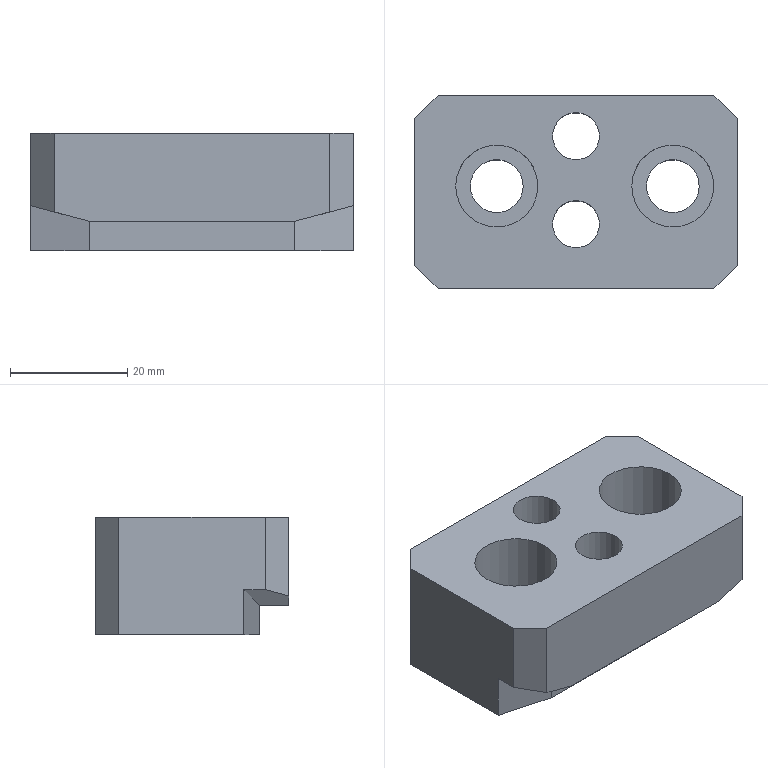Part | NX | features 20 2 | 1 solid | 24 faces | box 55 x 33 x 20 mm | volume 27724 mm3 | plane 18 | cylinder 6 | commonest cylinder face diameters 8.001 x2 9 x2 14 x2
STEP:
#1=CARTESIAN_POINT('',(974.002,435.,-3.5));
#2=VERTEX_POINT('',#1);
#3=CARTESIAN_POINT('',(969.502,435.,-3.5));
#4=DIRECTION('',(0.,0.,-1.));
#5=DIRECTION('',(1.,0.,0.));
#6=AXIS2_PLACEMENT_3D('',#3,#4,#5);
#7=CIRCLE('',#6,4.5);
#8=EDGE_CURVE('',#2,#2,#7,.T.);
#9=ORIENTED_EDGE('',*,*,#8,.F.);
#10=EDGE_LOOP('',(#9));
#11=FACE_BOUND('',#10,.T.);
#12=CARTESIAN_POINT('',(944.002,435.,-3.5));
#13=VERTEX_POINT('',#12);
#14=CARTESIAN_POINT('',(939.502,435.,-3.5));
#15=DIRECTION('',(0.,0.,1.));
#16=DIRECTION('',(1.,0.,0.));
#17=AXIS2_PLACEMENT_3D('',#14,#15,#16);
#18=CIRCLE('',#17,4.5);
#19=EDGE_CURVE('',#13,#13,#18,.T.);
#20=ORIENTED_EDGE('',*,*,#19,.T.);
#21=EDGE_LOOP('',(#20));
#22=FACE_BOUND('',#21,.T.);
#23=CARTESIAN_POINT('',(980.502,425.18,-3.5));
#24=VERTEX_POINT('',#23);
#25=CARTESIAN_POINT('',(970.501,422.5,-3.5));
#26=VERTEX_POINT('',#25);
#27=CARTESIAN_POINT('',(980.502,425.18,-3.5));
#28=DIRECTION('',(-0.9659,-0.2588,0.));
#29=VECTOR('',#28,1000.);
#30=LINE('',#27,#29);
#31=EDGE_CURVE('',#24,#26,#30,.T.);
#32=ORIENTED_EDGE('',*,*,#31,.T.);
#33=CARTESIAN_POINT('',(935.501,422.5,-3.5));
#34=VERTEX_POINT('',#33);
#35=CARTESIAN_POINT('',(981.501,422.5,-3.5));
#36=DIRECTION('',(-1.,0.,0.));
#37=VECTOR('',#36,1000.);
#38=LINE('',#35,#37);
#39=EDGE_CURVE('',#26,#34,#38,.T.);
#40=ORIENTED_EDGE('',*,*,#39,.T.);
#41=CARTESIAN_POINT('',(925.502,425.179,-3.5));
#42=VERTEX_POINT('',#41);
#43=CARTESIAN_POINT('',(935.501,422.5,-3.5));
#44=DIRECTION('',(-0.9659,0.2588,0.));
#45=VECTOR('',#44,1000.);
#46=LINE('',#43,#45);
#47=EDGE_CURVE('',#34,#42,#46,.T.);
#48=ORIENTED_EDGE('',*,*,#47,.T.);
#49=CARTESIAN_POINT('',(925.502,446.5,-3.5));
#50=VERTEX_POINT('',#49);
#51=CARTESIAN_POINT('',(925.502,417.5,-3.5));
#52=DIRECTION('',(0.,1.,0.));
#53=VECTOR('',#52,1000.);
#54=LINE('',#51,#53);
#55=EDGE_CURVE('',#42,#50,#54,.T.);
#56=ORIENTED_EDGE('',*,*,#55,.T.);
#57=CARTESIAN_POINT('',(929.502,450.5,-3.5));
#58=VERTEX_POINT('',#57);
#59=CARTESIAN_POINT('',(929.502,450.5,-3.5));
#60=DIRECTION('',(-0.7071,-0.7071,0.));
#61=VECTOR('',#60,1000.);
#62=LINE('',#59,#61);
#63=EDGE_CURVE('',#58,#50,#62,.T.);
#64=ORIENTED_EDGE('',*,*,#63,.F.);
#65=CARTESIAN_POINT('',(976.502,450.5,-3.5));
#66=VERTEX_POINT('',#65);
#67=CARTESIAN_POINT('',(1003.502,450.5,-3.5));
#68=DIRECTION('',(1.,0.,0.));
#69=VECTOR('',#68,1000.);
#70=LINE('',#67,#69);
#71=EDGE_CURVE('',#58,#66,#70,.T.);
#72=ORIENTED_EDGE('',*,*,#71,.T.);
#73=CARTESIAN_POINT('',(980.502,446.5,-3.5));
#74=VERTEX_POINT('',#73);
#75=CARTESIAN_POINT('',(980.502,446.5,-3.5));
#76=DIRECTION('',(-0.7071,0.7071,0.));
#77=VECTOR('',#76,1000.);
#78=LINE('',#75,#77);
#79=EDGE_CURVE('',#74,#66,#78,.T.);
#80=ORIENTED_EDGE('',*,*,#79,.F.);
#81=CARTESIAN_POINT('',(980.502,450.5,-3.5));
#82=DIRECTION('',(0.,-1.,0.));
#83=VECTOR('',#82,1000.);
#84=LINE('',#81,#83);
#85=EDGE_CURVE('',#74,#24,#84,.T.);
#86=ORIENTED_EDGE('',*,*,#85,.T.);
#87=EDGE_LOOP('',(#32,#40,#48,#56,#64,#72,#80,#86));
#88=FACE_BOUND('',#87,.T.);
#89=CARTESIAN_POINT('',(957.003,443.5,-3.5));
#90=VERTEX_POINT('',#89);
#91=CARTESIAN_POINT('',(953.002,443.5,-3.5));
#92=DIRECTION('',(0.,0.,1.));
#93=DIRECTION('',(1.,0.,0.));
#94=AXIS2_PLACEMENT_3D('',#91,#92,#93);
#95=CIRCLE('',#94,4.);
#96=EDGE_CURVE('',#90,#90,#95,.T.);
#97=ORIENTED_EDGE('',*,*,#96,.T.);
#98=EDGE_LOOP('',(#97));
#99=FACE_BOUND('',#98,.T.);
#100=CARTESIAN_POINT('',(957.003,428.5,-3.5));
#101=VERTEX_POINT('',#100);
#102=CARTESIAN_POINT('',(953.002,428.5,-3.5));
#103=DIRECTION('',(0.,0.,-1.));
#104=DIRECTION('',(1.,0.,0.));
#105=AXIS2_PLACEMENT_3D('',#102,#103,#104);
#106=CIRCLE('',#105,4.);
#107=EDGE_CURVE('',#101,#101,#106,.T.);
#108=ORIENTED_EDGE('',*,*,#107,.F.);
#109=EDGE_LOOP('',(#108));
#110=FACE_BOUND('',#109,.T.);
#111=CARTESIAN_POINT('',(1073.502,450.5,-3.5));
#112=DIRECTION('',(0.,0.,1.));
#113=DIRECTION('',(-1.,0.,0.));
#114=AXIS2_PLACEMENT_3D('',#111,#112,#113);
#115=PLANE('',#114);
#116=ADVANCED_FACE('',(#11,#22,#88,#99,#110),#115,.F.);
#117=CARTESIAN_POINT('',(935.502,417.5,1.5));
#118=VERTEX_POINT('',#117);
#119=CARTESIAN_POINT('',(970.502,417.5,1.5));
#120=VERTEX_POINT('',#119);
#121=CARTESIAN_POINT('',(1021.502,417.5,1.5));
#122=DIRECTION('',(1.,0.,0.));
#123=VECTOR('',#122,1000.);
#124=LINE('',#121,#123);
#125=EDGE_CURVE('',#118,#120,#124,.T.);
#126=ORIENTED_EDGE('',*,*,#125,.T.);
#127=CARTESIAN_POINT('',(976.502,417.5,3.108));
#128=VERTEX_POINT('',#127);
#129=CARTESIAN_POINT('',(970.502,417.5,1.5));
#130=DIRECTION('',(-0.9659,0.,-0.2588));
#131=VECTOR('',#130,1000.);
#132=LINE('',#129,#131);
#133=EDGE_CURVE('',#128,#120,#132,.T.);
#134=ORIENTED_EDGE('',*,*,#133,.F.);
#135=CARTESIAN_POINT('',(976.502,417.5,16.5));
#136=VERTEX_POINT('',#135);
#137=CARTESIAN_POINT('',(976.502,417.5,11.5));
#138=DIRECTION('',(0.,0.,-1.));
#139=VECTOR('',#138,1000.);
#140=LINE('',#137,#139);
#141=EDGE_CURVE('',#136,#128,#140,.T.);
#142=ORIENTED_EDGE('',*,*,#141,.F.);
#143=CARTESIAN_POINT('',(929.502,417.5,16.5));
#144=VERTEX_POINT('',#143);
#145=CARTESIAN_POINT('',(1043.502,417.5,16.5));
#146=DIRECTION('',(-1.,0.,0.));
#147=VECTOR('',#146,1000.);
#148=LINE('',#145,#147);
#149=EDGE_CURVE('',#136,#144,#148,.T.);
#150=ORIENTED_EDGE('',*,*,#149,.T.);
#151=CARTESIAN_POINT('',(929.502,417.5,3.108));
#152=VERTEX_POINT('',#151);
#153=CARTESIAN_POINT('',(929.502,417.5,11.5));
#154=DIRECTION('',(0.,0.,1.));
#155=VECTOR('',#154,1000.);
#156=LINE('',#153,#155);
#157=EDGE_CURVE('',#152,#144,#156,.T.);
#158=ORIENTED_EDGE('',*,*,#157,.F.);
#159=CARTESIAN_POINT('',(935.502,417.5,1.5));
#160=DIRECTION('',(-0.9659,0.,0.2588));
#161=VECTOR('',#160,1000.);
#162=LINE('',#159,#161);
#163=EDGE_CURVE('',#118,#152,#162,.T.);
#164=ORIENTED_EDGE('',*,*,#163,.F.);
#165=EDGE_LOOP('',(#126,#134,#142,#150,#158,#164));
#166=FACE_BOUND('',#165,.T.);
#167=CARTESIAN_POINT('',(1043.502,417.5,11.5));
#168=DIRECTION('',(0.,1.,0.));
#169=DIRECTION('',(0.,0.,1.));
#170=AXIS2_PLACEMENT_3D('',#167,#168,#169);
#171=PLANE('',#170);
#172=ADVANCED_FACE('',(#166),#171,.F.);
#173=CARTESIAN_POINT('',(957.003,428.5,16.5));
#174=VERTEX_POINT('',#173);
#175=CARTESIAN_POINT('',(953.002,428.5,16.5));
#176=DIRECTION('',(0.,0.,1.));
#177=DIRECTION('',(1.,0.,0.));
#178=AXIS2_PLACEMENT_3D('',#175,#176,#177);
#179=CIRCLE('',#178,4.);
#180=EDGE_CURVE('',#174,#174,#179,.T.);
#181=ORIENTED_EDGE('',*,*,#180,.F.);
#182=EDGE_LOOP('',(#181));
#183=FACE_BOUND('',#182,.T.);
#184=CARTESIAN_POINT('',(957.003,443.5,16.5));
#185=VERTEX_POINT('',#184);
#186=CARTESIAN_POINT('',(953.002,443.5,16.5));
#187=DIRECTION('',(0.,0.,1.));
#188=DIRECTION('',(1.,0.,0.));
#189=AXIS2_PLACEMENT_3D('',#186,#187,#188);
#190=CIRCLE('',#189,4.);
#191=EDGE_CURVE('',#185,#185,#190,.T.);
#192=ORIENTED_EDGE('',*,*,#191,.F.);
#193=EDGE_LOOP('',(#192));
#194=FACE_BOUND('',#193,.T.);
#195=CARTESIAN_POINT('',(976.502,435.,16.5));
#196=VERTEX_POINT('',#195);
#197=CARTESIAN_POINT('',(969.502,435.,16.5));
#198=DIRECTION('',(0.,0.,-1.));
#199=DIRECTION('',(1.,0.,0.));
#200=AXIS2_PLACEMENT_3D('',#197,#198,#199);
#201=CIRCLE('',#200,7.);
#202=EDGE_CURVE('',#196,#196,#201,.T.);
#203=ORIENTED_EDGE('',*,*,#202,.T.);
#204=EDGE_LOOP('',(#203));
#205=FACE_BOUND('',#204,.T.);
#206=CARTESIAN_POINT('',(946.502,435.,16.5));
#207=VERTEX_POINT('',#206);
#208=CARTESIAN_POINT('',(939.502,435.,16.5));
#209=DIRECTION('',(0.,0.,-1.));
#210=DIRECTION('',(1.,0.,0.));
#211=AXIS2_PLACEMENT_3D('',#208,#209,#210);
#212=CIRCLE('',#211,7.);
#213=EDGE_CURVE('',#207,#207,#212,.T.);
#214=ORIENTED_EDGE('',*,*,#213,.T.);
#215=EDGE_LOOP('',(#214));
#216=FACE_BOUND('',#215,.T.);
#217=ORIENTED_EDGE('',*,*,#149,.F.);
#218=CARTESIAN_POINT('',(980.502,421.5,16.5));
#219=VERTEX_POINT('',#218);
#220=CARTESIAN_POINT('',(976.502,417.5,16.5));
#221=DIRECTION('',(-0.7071,-0.7071,0.));
#222=VECTOR('',#221,1000.);
#223=LINE('',#220,#222);
#224=EDGE_CURVE('',#219,#136,#223,.T.);
#225=ORIENTED_EDGE('',*,*,#224,.F.);
#226=CARTESIAN_POINT('',(980.502,446.5,16.5));
#227=VERTEX_POINT('',#226);
#228=CARTESIAN_POINT('',(980.502,450.5,16.5));
#229=DIRECTION('',(0.,-1.,0.));
#230=VECTOR('',#229,1000.);
#231=LINE('',#228,#230);
#232=EDGE_CURVE('',#227,#219,#231,.T.);
#233=ORIENTED_EDGE('',*,*,#232,.F.);
#234=CARTESIAN_POINT('',(976.502,450.5,16.5));
#235=VERTEX_POINT('',#234);
#236=CARTESIAN_POINT('',(980.502,446.5,16.5));
#237=DIRECTION('',(0.7071,-0.7071,0.));
#238=VECTOR('',#237,1000.);
#239=LINE('',#236,#238);
#240=EDGE_CURVE('',#235,#227,#239,.T.);
#241=ORIENTED_EDGE('',*,*,#240,.F.);
#242=CARTESIAN_POINT('',(929.502,450.5,16.5));
#243=VERTEX_POINT('',#242);
#244=CARTESIAN_POINT('',(963.502,450.5,16.5));
#245=DIRECTION('',(1.,0.,0.));
#246=VECTOR('',#245,1000.);
#247=LINE('',#244,#246);
#248=EDGE_CURVE('',#243,#235,#247,.T.);
#249=ORIENTED_EDGE('',*,*,#248,.F.);
#250=CARTESIAN_POINT('',(925.502,446.5,16.5));
#251=VERTEX_POINT('',#250);
#252=CARTESIAN_POINT('',(929.502,450.5,16.5));
#253=DIRECTION('',(0.7071,0.7071,0.));
#254=VECTOR('',#253,1000.);
#255=LINE('',#252,#254);
#256=EDGE_CURVE('',#251,#243,#255,.T.);
#257=ORIENTED_EDGE('',*,*,#256,.F.);
#258=CARTESIAN_POINT('',(925.502,421.5,16.5));
#259=VERTEX_POINT('',#258);
#260=CARTESIAN_POINT('',(925.502,417.5,16.5));
#261=DIRECTION('',(0.,1.,0.));
#262=VECTOR('',#261,1000.);
#263=LINE('',#260,#262);
#264=EDGE_CURVE('',#259,#251,#263,.T.);
#265=ORIENTED_EDGE('',*,*,#264,.F.);
#266=CARTESIAN_POINT('',(925.502,421.5,16.5));
#267=DIRECTION('',(-0.7071,0.7071,0.));
#268=VECTOR('',#267,1000.);
#269=LINE('',#266,#268);
#270=EDGE_CURVE('',#144,#259,#269,.T.);
#271=ORIENTED_EDGE('',*,*,#270,.F.);
#272=EDGE_LOOP('',(#217,#225,#233,#241,#249,#257,#265,#271));
#273=FACE_BOUND('',#272,.T.);
#274=CARTESIAN_POINT('',(1043.502,450.5,16.5));
#275=DIRECTION('',(0.,0.,1.));
#276=DIRECTION('',(-1.,0.,0.));
#277=AXIS2_PLACEMENT_3D('',#274,#275,#276);
#278=PLANE('',#277);
#279=ADVANCED_FACE('',(#183,#194,#205,#216,#273),#278,.T.);
#280=CARTESIAN_POINT('',(965.002,435.,6.5));
#281=VERTEX_POINT('',#280);
#282=CARTESIAN_POINT('',(969.502,435.,6.5));
#283=DIRECTION('',(0.,0.,1.));
#284=DIRECTION('',(-1.,0.,0.));
#285=AXIS2_PLACEMENT_3D('',#282,#283,#284);
#286=CIRCLE('',#285,4.5);
#287=EDGE_CURVE('',#281,#281,#286,.T.);
#288=ORIENTED_EDGE('',*,*,#287,.F.);
#289=EDGE_LOOP('',(#288));
#290=FACE_BOUND('',#289,.T.);
#291=CARTESIAN_POINT('',(962.502,435.,6.5));
#292=VERTEX_POINT('',#291);
#293=CARTESIAN_POINT('',(969.502,435.,6.5));
#294=DIRECTION('',(0.,0.,-1.));
#295=DIRECTION('',(-1.,0.,0.));
#296=AXIS2_PLACEMENT_3D('',#293,#294,#295);
#297=CIRCLE('',#296,7.);
#298=EDGE_CURVE('',#292,#292,#297,.T.);
#299=ORIENTED_EDGE('',*,*,#298,.F.);
#300=EDGE_LOOP('',(#299));
#301=FACE_BOUND('',#300,.T.);
#302=CARTESIAN_POINT('',(969.502,432.5,6.5));
#303=DIRECTION('',(0.,0.,-1.));
#304=DIRECTION('',(1.,0.,0.));
#305=AXIS2_PLACEMENT_3D('',#302,#303,#304);
#306=PLANE('',#305);
#307=ADVANCED_FACE('',(#290,#301),#306,.F.);
#308=CARTESIAN_POINT('',(970.502,422.5,1.5));
#309=VERTEX_POINT('',#308);
#310=CARTESIAN_POINT('',(970.502,425.18,1.5));
#311=DIRECTION('',(0.,1.,0.));
#312=VECTOR('',#311,1000.);
#313=LINE('',#310,#312);
#314=EDGE_CURVE('',#120,#309,#313,.T.);
#315=ORIENTED_EDGE('',*,*,#314,.T.);
#316=CARTESIAN_POINT('',(980.502,425.18,4.179));
#317=VERTEX_POINT('',#316);
#318=CARTESIAN_POINT('',(979.875,425.012,4.011));
#319=DIRECTION('',(0.9351,0.2506,0.2506));
#320=VECTOR('',#319,1000.);
#321=LINE('',#318,#320);
#322=EDGE_CURVE('',#309,#317,#321,.T.);
#323=ORIENTED_EDGE('',*,*,#322,.T.);
#324=CARTESIAN_POINT('',(980.502,421.5,4.179));
#325=VERTEX_POINT('',#324);
#326=CARTESIAN_POINT('',(980.502,417.5,4.179));
#327=DIRECTION('',(0.,-1.,0.));
#328=VECTOR('',#327,1000.);
#329=LINE('',#326,#328);
#330=EDGE_CURVE('',#317,#325,#329,.T.);
#331=ORIENTED_EDGE('',*,*,#330,.T.);
#332=CARTESIAN_POINT('',(963.451,404.449,-0.3894));
#333=DIRECTION('',(0.6947,0.6947,0.1862));
#334=VECTOR('',#333,1000.);
#335=LINE('',#332,#334);
#336=EDGE_CURVE('',#128,#325,#335,.T.);
#337=ORIENTED_EDGE('',*,*,#336,.F.);
#338=ORIENTED_EDGE('',*,*,#133,.T.);
#339=EDGE_LOOP('',(#315,#323,#331,#337,#338));
#340=FACE_BOUND('',#339,.T.);
#341=CARTESIAN_POINT('',(970.502,396.891,1.5));
#342=DIRECTION('',(0.2588,0.,-0.9659));
#343=DIRECTION('',(0.9659,0.,0.2588));
#344=AXIS2_PLACEMENT_3D('',#341,#342,#343);
#345=PLANE('',#344);
#346=ADVANCED_FACE('',(#340),#345,.T.);
#347=CARTESIAN_POINT('',(935.002,435.,6.5));
#348=VERTEX_POINT('',#347);
#349=CARTESIAN_POINT('',(939.502,435.,6.5));
#350=DIRECTION('',(0.,0.,1.));
#351=DIRECTION('',(-1.,0.,0.));
#352=AXIS2_PLACEMENT_3D('',#349,#350,#351);
#353=CIRCLE('',#352,4.5);
#354=EDGE_CURVE('',#348,#348,#353,.T.);
#355=ORIENTED_EDGE('',*,*,#354,.F.);
#356=EDGE_LOOP('',(#355));
#357=FACE_BOUND('',#356,.T.);
#358=CARTESIAN_POINT('',(932.502,435.,6.5));
#359=VERTEX_POINT('',#358);
#360=CARTESIAN_POINT('',(939.502,435.,6.5));
#361=DIRECTION('',(0.,0.,-1.));
#362=DIRECTION('',(-1.,0.,0.));
#363=AXIS2_PLACEMENT_3D('',#360,#361,#362);
#364=CIRCLE('',#363,7.);
#365=EDGE_CURVE('',#359,#359,#364,.T.);
#366=ORIENTED_EDGE('',*,*,#365,.F.);
#367=EDGE_LOOP('',(#366));
#368=FACE_BOUND('',#367,.T.);
#369=CARTESIAN_POINT('',(939.502,432.5,6.5));
#370=DIRECTION('',(0.,0.,-1.));
#371=DIRECTION('',(-1.,0.,0.));
#372=AXIS2_PLACEMENT_3D('',#369,#370,#371);
#373=PLANE('',#372);
#374=ADVANCED_FACE('',(#357,#368),#373,.F.);
#375=ORIENTED_EDGE('',*,*,#202,.F.);
#376=EDGE_LOOP('',(#375));
#377=FACE_BOUND('',#376,.T.);
#378=ORIENTED_EDGE('',*,*,#298,.T.);
#379=EDGE_LOOP('',(#378));
#380=FACE_BOUND('',#379,.T.);
#381=CARTESIAN_POINT('',(969.502,435.,42.5));
#382=DIRECTION('',(0.,0.,-1.));
#383=DIRECTION('',(1.,0.,0.));
#384=AXIS2_PLACEMENT_3D('',#381,#382,#383);
#385=CYLINDRICAL_SURFACE('',#384,7.);
#386=ADVANCED_FACE('',(#377,#380),#385,.F.);
#387=ORIENTED_EDGE('',*,*,#224,.T.);
#388=ORIENTED_EDGE('',*,*,#141,.T.);
#389=ORIENTED_EDGE('',*,*,#336,.T.);
#390=CARTESIAN_POINT('',(980.502,421.5,11.5));
#391=DIRECTION('',(0.,0.,1.));
#392=VECTOR('',#391,1000.);
#393=LINE('',#390,#392);
#394=EDGE_CURVE('',#325,#219,#393,.T.);
#395=ORIENTED_EDGE('',*,*,#394,.T.);
#396=EDGE_LOOP('',(#387,#388,#389,#395));
#397=FACE_BOUND('',#396,.T.);
#398=CARTESIAN_POINT('',(976.502,417.5,11.5));
#399=DIRECTION('',(-0.7071,0.7071,0.));
#400=DIRECTION('',(0.,0.,-1.));
#401=AXIS2_PLACEMENT_3D('',#398,#399,#400);
#402=PLANE('',#401);
#403=ADVANCED_FACE('',(#397),#402,.F.);
#404=ORIENTED_EDGE('',*,*,#365,.T.);
#405=EDGE_LOOP('',(#404));
#406=FACE_BOUND('',#405,.T.);
#407=ORIENTED_EDGE('',*,*,#213,.F.);
#408=EDGE_LOOP('',(#407));
#409=FACE_BOUND('',#408,.T.);
#410=CARTESIAN_POINT('',(939.502,435.,42.5));
#411=DIRECTION('',(0.,0.,-1.));
#412=DIRECTION('',(-1.,0.,0.));
#413=AXIS2_PLACEMENT_3D('',#410,#411,#412);
#414=CYLINDRICAL_SURFACE('',#413,7.);
#415=ADVANCED_FACE('',(#406,#409),#414,.F.);
#416=ORIENTED_EDGE('',*,*,#330,.F.);
#417=CARTESIAN_POINT('',(980.502,425.18,3.5));
#418=DIRECTION('',(0.,0.,-1.));
#419=VECTOR('',#418,1000.);
#420=LINE('',#417,#419);
#421=EDGE_CURVE('',#317,#24,#420,.T.);
#422=ORIENTED_EDGE('',*,*,#421,.T.);
#423=ORIENTED_EDGE('',*,*,#85,.F.);
#424=CARTESIAN_POINT('',(980.502,446.5,11.5));
#425=DIRECTION('',(0.,0.,-1.));
#426=VECTOR('',#425,1000.);
#427=LINE('',#424,#426);
#428=EDGE_CURVE('',#227,#74,#427,.T.);
#429=ORIENTED_EDGE('',*,*,#428,.F.);
#430=ORIENTED_EDGE('',*,*,#232,.T.);
#431=ORIENTED_EDGE('',*,*,#394,.F.);
#432=EDGE_LOOP('',(#416,#422,#423,#429,#430,#431));
#433=FACE_BOUND('',#432,.T.);
#434=CARTESIAN_POINT('',(980.502,450.5,11.5));
#435=DIRECTION('',(-1.,0.,0.));
#436=DIRECTION('',(0.,0.,-1.));
#437=AXIS2_PLACEMENT_3D('',#434,#435,#436);
#438=PLANE('',#437);
#439=ADVANCED_FACE('',(#433),#438,.F.);
#440=CARTESIAN_POINT('',(970.501,422.5,1.5));
#441=VERTEX_POINT('',#440);
#442=CARTESIAN_POINT('',(980.502,425.18,1.5));
#443=DIRECTION('',(0.9659,0.2588,0.));
#444=VECTOR('',#443,1000.);
#445=LINE('',#442,#444);
#446=EDGE_CURVE('',#441,#309,#445,.T.);
#447=ORIENTED_EDGE('',*,*,#446,.F.);
#448=CARTESIAN_POINT('',(970.501,422.5,3.5));
#449=DIRECTION('',(0.,0.,1.));
#450=VECTOR('',#449,1000.);
#451=LINE('',#448,#450);
#452=EDGE_CURVE('',#26,#441,#451,.T.);
#453=ORIENTED_EDGE('',*,*,#452,.F.);
#454=ORIENTED_EDGE('',*,*,#31,.F.);
#455=ORIENTED_EDGE('',*,*,#421,.F.);
#456=ORIENTED_EDGE('',*,*,#322,.F.);
#457=EDGE_LOOP('',(#447,#453,#454,#455,#456));
#458=FACE_BOUND('',#457,.T.);
#459=CARTESIAN_POINT('',(980.502,425.18,3.5));
#460=DIRECTION('',(-0.2588,0.9659,0.));
#461=DIRECTION('',(0.9659,0.2588,0.));
#462=AXIS2_PLACEMENT_3D('',#459,#460,#461);
#463=PLANE('',#462);
#464=ADVANCED_FACE('',(#458),#463,.F.);
#465=ORIENTED_EDGE('',*,*,#287,.T.);
#466=EDGE_LOOP('',(#465));
#467=FACE_BOUND('',#466,.T.);
#468=ORIENTED_EDGE('',*,*,#8,.T.);
#469=EDGE_LOOP('',(#468));
#470=FACE_BOUND('',#469,.T.);
#471=CARTESIAN_POINT('',(969.502,435.,42.5));
#472=DIRECTION('',(0.,0.,-1.));
#473=DIRECTION('',(1.,0.,0.));
#474=AXIS2_PLACEMENT_3D('',#471,#472,#473);
#475=CYLINDRICAL_SURFACE('',#474,4.5);
#476=ADVANCED_FACE('',(#467,#470),#475,.F.);
#477=CARTESIAN_POINT('',(925.502,421.5,4.179));
#478=VERTEX_POINT('',#477);
#479=CARTESIAN_POINT('',(925.502,421.5,11.5));
#480=DIRECTION('',(0.,0.,-1.));
#481=VECTOR('',#480,1000.);
#482=LINE('',#479,#481);
#483=EDGE_CURVE('',#259,#478,#482,.T.);
#484=ORIENTED_EDGE('',*,*,#483,.T.);
#485=CARTESIAN_POINT('',(942.554,404.449,-0.3894));
#486=DIRECTION('',(0.6947,-0.6947,-0.1862));
#487=VECTOR('',#486,1000.);
#488=LINE('',#485,#487);
#489=EDGE_CURVE('',#478,#152,#488,.T.);
#490=ORIENTED_EDGE('',*,*,#489,.T.);
#491=ORIENTED_EDGE('',*,*,#157,.T.);
#492=ORIENTED_EDGE('',*,*,#270,.T.);
#493=EDGE_LOOP('',(#484,#490,#491,#492));
#494=FACE_BOUND('',#493,.T.);
#495=CARTESIAN_POINT('',(925.502,421.5,11.5));
#496=DIRECTION('',(0.7071,0.7071,0.));
#497=DIRECTION('',(0.,0.,-1.));
#498=AXIS2_PLACEMENT_3D('',#495,#496,#497);
#499=PLANE('',#498);
#500=ADVANCED_FACE('',(#494),#499,.F.);
#501=ORIENTED_EDGE('',*,*,#19,.F.);
#502=EDGE_LOOP('',(#501));
#503=FACE_BOUND('',#502,.T.);
#504=ORIENTED_EDGE('',*,*,#354,.T.);
#505=EDGE_LOOP('',(#504));
#506=FACE_BOUND('',#505,.T.);
#507=CARTESIAN_POINT('',(939.502,435.,42.5));
#508=DIRECTION('',(0.,0.,-1.));
#509=DIRECTION('',(-1.,0.,0.));
#510=AXIS2_PLACEMENT_3D('',#507,#508,#509);
#511=CYLINDRICAL_SURFACE('',#510,4.5);
#512=ADVANCED_FACE('',(#503,#506),#511,.F.);
#513=ORIENTED_EDGE('',*,*,#55,.F.);
#514=CARTESIAN_POINT('',(925.502,425.179,4.179));
#515=VERTEX_POINT('',#514);
#516=CARTESIAN_POINT('',(925.502,425.179,3.5));
#517=DIRECTION('',(0.,0.,-1.));
#518=VECTOR('',#517,1000.);
#519=LINE('',#516,#518);
#520=EDGE_CURVE('',#515,#42,#519,.T.);
#521=ORIENTED_EDGE('',*,*,#520,.F.);
#522=CARTESIAN_POINT('',(925.502,425.179,4.179));
#523=DIRECTION('',(0.,1.,0.));
#524=VECTOR('',#523,1000.);
#525=LINE('',#522,#524);
#526=EDGE_CURVE('',#478,#515,#525,.T.);
#527=ORIENTED_EDGE('',*,*,#526,.F.);
#528=ORIENTED_EDGE('',*,*,#483,.F.);
#529=ORIENTED_EDGE('',*,*,#264,.T.);
#530=CARTESIAN_POINT('',(925.502,446.5,11.5));
#531=DIRECTION('',(0.,0.,1.));
#532=VECTOR('',#531,1000.);
#533=LINE('',#530,#532);
#534=EDGE_CURVE('',#50,#251,#533,.T.);
#535=ORIENTED_EDGE('',*,*,#534,.F.);
#536=EDGE_LOOP('',(#513,#521,#527,#528,#529,#535));
#537=FACE_BOUND('',#536,.T.);
#538=CARTESIAN_POINT('',(925.502,417.5,11.5));
#539=DIRECTION('',(1.,0.,0.));
#540=DIRECTION('',(0.,0.,1.));
#541=AXIS2_PLACEMENT_3D('',#538,#539,#540);
#542=PLANE('',#541);
#543=ADVANCED_FACE('',(#537),#542,.F.);
#544=ORIENTED_EDGE('',*,*,#526,.T.);
#545=CARTESIAN_POINT('',(935.501,422.5,1.5));
#546=VERTEX_POINT('',#545);
#547=CARTESIAN_POINT('',(935.501,422.5,1.5));
#548=DIRECTION('',(0.9351,-0.2506,-0.2506));
#549=VECTOR('',#548,1000.);
#550=LINE('',#547,#549);
#551=EDGE_CURVE('',#515,#546,#550,.T.);
#552=ORIENTED_EDGE('',*,*,#551,.T.);
#553=CARTESIAN_POINT('',(935.502,422.5,1.5));
#554=VERTEX_POINT('',#553);
#555=CARTESIAN_POINT('',(935.502,422.5,1.5));
#556=DIRECTION('',(0.9659,0.,-0.2588));
#557=VECTOR('',#556,1000.);
#558=LINE('',#555,#557);
#559=EDGE_CURVE('',#546,#554,#558,.T.);
#560=ORIENTED_EDGE('',*,*,#559,.T.);
#561=CARTESIAN_POINT('',(935.502,417.5,1.5));
#562=DIRECTION('',(0.,-1.,0.));
#563=VECTOR('',#562,1000.);
#564=LINE('',#561,#563);
#565=EDGE_CURVE('',#554,#118,#564,.T.);
#566=ORIENTED_EDGE('',*,*,#565,.T.);
#567=ORIENTED_EDGE('',*,*,#163,.T.);
#568=ORIENTED_EDGE('',*,*,#489,.F.);
#569=EDGE_LOOP('',(#544,#552,#560,#566,#567,#568));
#570=FACE_BOUND('',#569,.T.);
#571=CARTESIAN_POINT('',(935.502,396.891,1.5));
#572=DIRECTION('',(-0.2588,0.,-0.9659));
#573=DIRECTION('',(0.9659,0.,-0.2588));
#574=AXIS2_PLACEMENT_3D('',#571,#572,#573);
#575=PLANE('',#574);
#576=ADVANCED_FACE('',(#570),#575,.T.);
#577=ORIENTED_EDGE('',*,*,#47,.F.);
#578=CARTESIAN_POINT('',(935.501,422.5,3.5));
#579=DIRECTION('',(0.,0.,1.));
#580=VECTOR('',#579,1000.);
#581=LINE('',#578,#580);
#582=EDGE_CURVE('',#34,#546,#581,.T.);
#583=ORIENTED_EDGE('',*,*,#582,.T.);
#584=ORIENTED_EDGE('',*,*,#551,.F.);
#585=ORIENTED_EDGE('',*,*,#520,.T.);
#586=EDGE_LOOP('',(#577,#583,#584,#585));
#587=FACE_BOUND('',#586,.T.);
#588=CARTESIAN_POINT('',(935.501,422.5,3.5));
#589=DIRECTION('',(0.2588,0.9659,0.));
#590=DIRECTION('',(0.9659,-0.2588,0.));
#591=AXIS2_PLACEMENT_3D('',#588,#589,#590);
#592=PLANE('',#591);
#593=ADVANCED_FACE('',(#587),#592,.F.);
#594=ORIENTED_EDGE('',*,*,#63,.T.);
#595=ORIENTED_EDGE('',*,*,#534,.T.);
#596=ORIENTED_EDGE('',*,*,#256,.T.);
#597=CARTESIAN_POINT('',(929.502,450.5,11.5));
#598=DIRECTION('',(0.,0.,-1.));
#599=VECTOR('',#598,1000.);
#600=LINE('',#597,#599);
#601=EDGE_CURVE('',#243,#58,#600,.T.);
#602=ORIENTED_EDGE('',*,*,#601,.T.);
#603=EDGE_LOOP('',(#594,#595,#596,#602));
#604=FACE_BOUND('',#603,.T.);
#605=CARTESIAN_POINT('',(929.502,450.5,11.5));
#606=DIRECTION('',(0.7071,-0.7071,0.));
#607=DIRECTION('',(0.,0.,-1.));
#608=AXIS2_PLACEMENT_3D('',#605,#606,#607);
#609=PLANE('',#608);
#610=ADVANCED_FACE('',(#604),#609,.F.);
#611=ORIENTED_EDGE('',*,*,#79,.T.);
#612=CARTESIAN_POINT('',(976.502,450.5,11.5));
#613=DIRECTION('',(0.,0.,1.));
#614=VECTOR('',#613,1000.);
#615=LINE('',#612,#614);
#616=EDGE_CURVE('',#66,#235,#615,.T.);
#617=ORIENTED_EDGE('',*,*,#616,.T.);
#618=ORIENTED_EDGE('',*,*,#240,.T.);
#619=ORIENTED_EDGE('',*,*,#428,.T.);
#620=EDGE_LOOP('',(#611,#617,#618,#619));
#621=FACE_BOUND('',#620,.T.);
#622=CARTESIAN_POINT('',(980.502,446.5,11.5));
#623=DIRECTION('',(-0.7071,-0.7071,0.));
#624=DIRECTION('',(0.,0.,-1.));
#625=AXIS2_PLACEMENT_3D('',#622,#623,#624);
#626=PLANE('',#625);
#627=ADVANCED_FACE('',(#621),#626,.F.);
#628=ORIENTED_EDGE('',*,*,#71,.F.);
#629=ORIENTED_EDGE('',*,*,#601,.F.);
#630=ORIENTED_EDGE('',*,*,#248,.T.);
#631=ORIENTED_EDGE('',*,*,#616,.F.);
#632=EDGE_LOOP('',(#628,#629,#630,#631));
#633=FACE_BOUND('',#632,.T.);
#634=CARTESIAN_POINT('',(963.502,450.5,11.5));
#635=DIRECTION('',(0.,-1.,0.));
#636=DIRECTION('',(0.,0.,-1.));
#637=AXIS2_PLACEMENT_3D('',#634,#635,#636);
#638=PLANE('',#637);
#639=ADVANCED_FACE('',(#633),#638,.F.);
#640=ORIENTED_EDGE('',*,*,#125,.F.);
#641=ORIENTED_EDGE('',*,*,#565,.F.);
#642=CARTESIAN_POINT('',(1011.501,422.5,1.5));
#643=DIRECTION('',(1.,0.,0.));
#644=VECTOR('',#643,1000.);
#645=LINE('',#642,#644);
#646=EDGE_CURVE('',#554,#441,#645,.T.);
#647=ORIENTED_EDGE('',*,*,#646,.T.);
#648=ORIENTED_EDGE('',*,*,#446,.T.);
#649=ORIENTED_EDGE('',*,*,#314,.F.);
#650=EDGE_LOOP('',(#640,#641,#647,#648,#649));
#651=FACE_BOUND('',#650,.T.);
#652=CARTESIAN_POINT('',(1043.773,396.891,1.5));
#653=DIRECTION('',(0.,0.,-1.));
#654=DIRECTION('',(1.,0.,0.));
#655=AXIS2_PLACEMENT_3D('',#652,#653,#654);
#656=PLANE('',#655);
#657=ADVANCED_FACE('',(#651),#656,.T.);
#658=ORIENTED_EDGE('',*,*,#646,.F.);
#659=ORIENTED_EDGE('',*,*,#559,.F.);
#660=ORIENTED_EDGE('',*,*,#582,.F.);
#661=ORIENTED_EDGE('',*,*,#39,.F.);
#662=ORIENTED_EDGE('',*,*,#452,.T.);
#663=EDGE_LOOP('',(#658,#659,#660,#661,#662));
#664=FACE_BOUND('',#663,.T.);
#665=CARTESIAN_POINT('',(1011.501,422.5,3.5));
#666=DIRECTION('',(0.,1.,0.));
#667=DIRECTION('',(0.,0.,1.));
#668=AXIS2_PLACEMENT_3D('',#665,#666,#667);
#669=PLANE('',#668);
#670=ADVANCED_FACE('',(#664),#669,.F.);
#671=ORIENTED_EDGE('',*,*,#191,.T.);
#672=EDGE_LOOP('',(#671));
#673=FACE_BOUND('',#672,.T.);
#674=ORIENTED_EDGE('',*,*,#96,.F.);
#675=EDGE_LOOP('',(#674));
#676=FACE_BOUND('',#675,.T.);
#677=CARTESIAN_POINT('',(953.002,443.5,-3.5));
#678=DIRECTION('',(0.,0.,1.));
#679=DIRECTION('',(-1.,0.,0.));
#680=AXIS2_PLACEMENT_3D('',#677,#678,#679);
#681=CYLINDRICAL_SURFACE('',#680,4.);
#682=ADVANCED_FACE('',(#673,#676),#681,.F.);
#683=ORIENTED_EDGE('',*,*,#180,.T.);
#684=EDGE_LOOP('',(#683));
#685=FACE_BOUND('',#684,.T.);
#686=ORIENTED_EDGE('',*,*,#107,.T.);
#687=EDGE_LOOP('',(#686));
#688=FACE_BOUND('',#687,.T.);
#689=CARTESIAN_POINT('',(953.002,428.5,-3.5));
#690=DIRECTION('',(0.,0.,1.));
#691=DIRECTION('',(-1.,0.,0.));
#692=AXIS2_PLACEMENT_3D('',#689,#690,#691);
#693=CYLINDRICAL_SURFACE('',#692,4.);
#694=ADVANCED_FACE('',(#685,#688),#693,.F.);
#695=CLOSED_SHELL('',(#116,#172,#279,#307,#346,#374,#386,#403,#415,#439,#464,#476,#500,#512,#543,#576,#593,#610,#627,#639,#657,#670,#682,#694));
#696=MANIFOLD_SOLID_BREP('',#695);
#697=(LENGTH_UNIT()NAMED_UNIT(*)SI_UNIT(.MILLI.,.METRE.));
#698=UNCERTAINTY_MEASURE_WITH_UNIT(LENGTH_MEASURE(0.00001),#697,'','');
#699=(NAMED_UNIT(*)PLANE_ANGLE_UNIT()SI_UNIT($,.RADIAN.));
#700=(NAMED_UNIT(*)SI_UNIT($,.STERADIAN.)SOLID_ANGLE_UNIT());
#701=(GEOMETRIC_REPRESENTATION_CONTEXT(3)GLOBAL_UNCERTAINTY_ASSIGNED_CONTEXT((#698))GLOBAL_UNIT_ASSIGNED_CONTEXT((#697,#699,#700))REPRESENTATION_CONTEXT('',''));
#702=ADVANCED_BREP_SHAPE_REPRESENTATION('',(#696),#701);